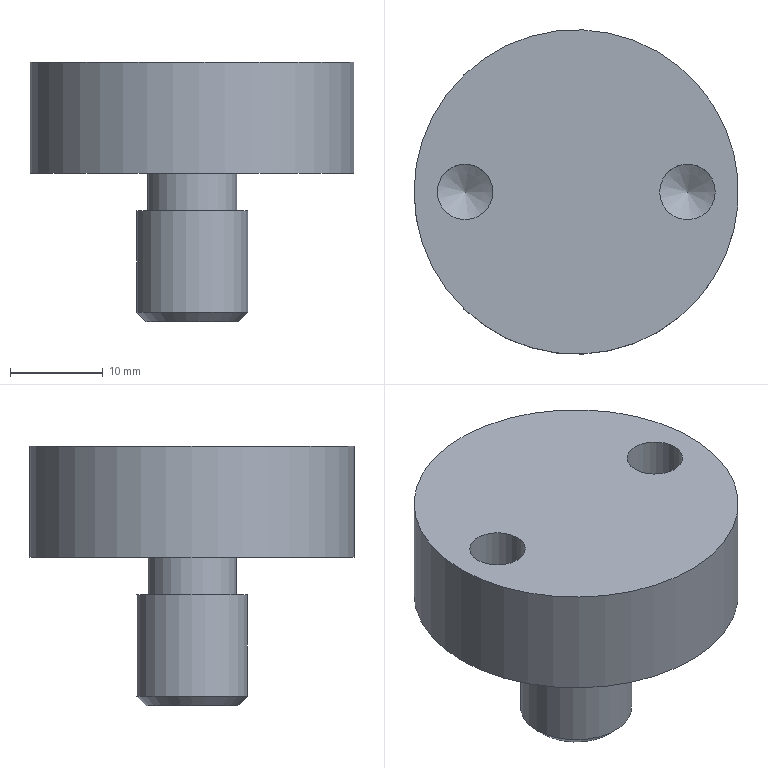Part | NX | features DATUM_CSYS 3, SIMPLE HOLE 2, SKETCH 2, CHAMFER 1, HOLE PACKAGE 1, SWP104 1, SYMBOLIC_THREAD 1 | 1 solid | 12 faces | box 35 x 35 x 28 mm | volume 12801 mm3 | cylinder 5 | plane 4 | cone 3 | commonest cylinder face diameters 6 x2 9.6 x1 12 x1 35 x1
STEP:
#1=CARTESIAN_POINT('',(-5.,0.,-28.));
#2=VERTEX_POINT('',#1);
#3=CARTESIAN_POINT('',(0.,0.,-28.));
#4=DIRECTION('',(0.,0.,-1.));
#5=DIRECTION('',(-1.,0.,0.));
#6=AXIS2_PLACEMENT_3D('',#3,#4,#5);
#7=CIRCLE('',#6,5.);
#8=EDGE_CURVE('',#2,#2,#7,.T.);
#9=ORIENTED_EDGE('',*,*,#8,.T.);
#10=EDGE_LOOP('',(#9));
#11=FACE_BOUND('',#10,.T.);
#12=CARTESIAN_POINT('',(0.,0.,-28.));
#13=DIRECTION('',(0.,0.,-1.));
#14=DIRECTION('',(-1.,0.,0.));
#15=AXIS2_PLACEMENT_3D('',#12,#13,#14);
#16=PLANE('',#15);
#17=ADVANCED_FACE('',(#11),#16,.T.);
#18=CARTESIAN_POINT('',(-6.,0.,-27.));
#19=VERTEX_POINT('',#18);
#20=CARTESIAN_POINT('',(0.,0.,-27.));
#21=DIRECTION('',(0.,0.,-1.));
#22=DIRECTION('',(-1.,0.,0.));
#23=AXIS2_PLACEMENT_3D('',#20,#21,#22);
#24=CIRCLE('',#23,6.);
#25=EDGE_CURVE('',#19,#19,#24,.F.);
#26=ORIENTED_EDGE('',*,*,#25,.T.);
#27=EDGE_LOOP('',(#26));
#28=FACE_BOUND('',#27,.T.);
#29=CARTESIAN_POINT('',(-6.,0.,-16.));
#30=VERTEX_POINT('',#29);
#31=CARTESIAN_POINT('',(0.,0.,-16.));
#32=DIRECTION('',(0.,0.,-1.));
#33=DIRECTION('',(-1.,0.,0.));
#34=AXIS2_PLACEMENT_3D('',#31,#32,#33);
#35=CIRCLE('',#34,6.);
#36=EDGE_CURVE('',#30,#30,#35,.T.);
#37=ORIENTED_EDGE('',*,*,#36,.T.);
#38=EDGE_LOOP('',(#37));
#39=FACE_BOUND('',#38,.T.);
#40=CARTESIAN_POINT('',(0.,0.,0.));
#41=DIRECTION('',(0.,0.,-1.));
#42=DIRECTION('',(-1.,0.,0.));
#43=AXIS2_PLACEMENT_3D('',#40,#41,#42);
#44=CYLINDRICAL_SURFACE('',#43,6.);
#45=ADVANCED_FACE('',(#28,#39),#44,.T.);
#46=CARTESIAN_POINT('',(-4.8,0.,-16.));
#47=VERTEX_POINT('',#46);
#48=CARTESIAN_POINT('',(0.,0.,-16.));
#49=DIRECTION('',(0.,0.,-1.));
#50=DIRECTION('',(-1.,0.,0.));
#51=AXIS2_PLACEMENT_3D('',#48,#49,#50);
#52=CIRCLE('',#51,4.8);
#53=EDGE_CURVE('',#47,#47,#52,.T.);
#54=ORIENTED_EDGE('',*,*,#53,.T.);
#55=EDGE_LOOP('',(#54));
#56=FACE_BOUND('',#55,.T.);
#57=ORIENTED_EDGE('',*,*,#36,.F.);
#58=EDGE_LOOP('',(#57));
#59=FACE_BOUND('',#58,.T.);
#60=CARTESIAN_POINT('',(6.,0.,-16.));
#61=DIRECTION('',(0.,0.,1.));
#62=DIRECTION('',(1.,0.,0.));
#63=AXIS2_PLACEMENT_3D('',#60,#61,#62);
#64=PLANE('',#63);
#65=ADVANCED_FACE('',(#56,#59),#64,.T.);
#66=CARTESIAN_POINT('',(-4.8,0.,-12.));
#67=VERTEX_POINT('',#66);
#68=CARTESIAN_POINT('',(0.,0.,-12.));
#69=DIRECTION('',(0.,0.,-1.));
#70=DIRECTION('',(-1.,0.,0.));
#71=AXIS2_PLACEMENT_3D('',#68,#69,#70);
#72=CIRCLE('',#71,4.8);
#73=EDGE_CURVE('',#67,#67,#72,.T.);
#74=ORIENTED_EDGE('',*,*,#73,.T.);
#75=EDGE_LOOP('',(#74));
#76=FACE_BOUND('',#75,.T.);
#77=ORIENTED_EDGE('',*,*,#53,.F.);
#78=EDGE_LOOP('',(#77));
#79=FACE_BOUND('',#78,.T.);
#80=CARTESIAN_POINT('',(0.,0.,0.));
#81=DIRECTION('',(0.,0.,-1.));
#82=DIRECTION('',(-1.,0.,0.));
#83=AXIS2_PLACEMENT_3D('',#80,#81,#82);
#84=CYLINDRICAL_SURFACE('',#83,4.8);
#85=ADVANCED_FACE('',(#76,#79),#84,.T.);
#86=CARTESIAN_POINT('',(-17.5,0.,-12.));
#87=VERTEX_POINT('',#86);
#88=CARTESIAN_POINT('',(0.,0.,-12.));
#89=DIRECTION('',(0.,0.,-1.));
#90=DIRECTION('',(-1.,0.,0.));
#91=AXIS2_PLACEMENT_3D('',#88,#89,#90);
#92=CIRCLE('',#91,17.5);
#93=EDGE_CURVE('',#87,#87,#92,.T.);
#94=ORIENTED_EDGE('',*,*,#93,.T.);
#95=EDGE_LOOP('',(#94));
#96=FACE_BOUND('',#95,.T.);
#97=ORIENTED_EDGE('',*,*,#73,.F.);
#98=EDGE_LOOP('',(#97));
#99=FACE_BOUND('',#98,.T.);
#100=CARTESIAN_POINT('',(4.8,0.,-12.));
#101=DIRECTION('',(0.,0.,-1.));
#102=DIRECTION('',(-1.,0.,0.));
#103=AXIS2_PLACEMENT_3D('',#100,#101,#102);
#104=PLANE('',#103);
#105=ADVANCED_FACE('',(#96,#99),#104,.T.);
#106=CARTESIAN_POINT('',(-17.5,0.,0.));
#107=VERTEX_POINT('',#106);
#108=CARTESIAN_POINT('',(0.,0.,0.));
#109=DIRECTION('',(0.,0.,-1.));
#110=DIRECTION('',(-1.,0.,0.));
#111=AXIS2_PLACEMENT_3D('',#108,#109,#110);
#112=CIRCLE('',#111,17.5);
#113=EDGE_CURVE('',#107,#107,#112,.T.);
#114=ORIENTED_EDGE('',*,*,#113,.T.);
#115=EDGE_LOOP('',(#114));
#116=FACE_BOUND('',#115,.T.);
#117=ORIENTED_EDGE('',*,*,#93,.F.);
#118=EDGE_LOOP('',(#117));
#119=FACE_BOUND('',#118,.T.);
#120=CARTESIAN_POINT('',(0.,0.,0.));
#121=DIRECTION('',(0.,0.,-1.));
#122=DIRECTION('',(-1.,0.,0.));
#123=AXIS2_PLACEMENT_3D('',#120,#121,#122);
#124=CYLINDRICAL_SURFACE('',#123,17.5);
#125=ADVANCED_FACE('',(#116,#119),#124,.T.);
#126=CARTESIAN_POINT('',(9.,0.,0.));
#127=VERTEX_POINT('',#126);
#128=CARTESIAN_POINT('',(12.,0.,0.));
#129=DIRECTION('',(0.,0.,-1.));
#130=DIRECTION('',(-1.,0.,0.));
#131=AXIS2_PLACEMENT_3D('',#128,#129,#130);
#132=CIRCLE('',#131,3.);
#133=EDGE_CURVE('',#127,#127,#132,.T.);
#134=ORIENTED_EDGE('',*,*,#133,.T.);
#135=EDGE_LOOP('',(#134));
#136=FACE_BOUND('',#135,.T.);
#137=CARTESIAN_POINT('',(-15.,0.,0.));
#138=VERTEX_POINT('',#137);
#139=CARTESIAN_POINT('',(-12.,0.,0.));
#140=DIRECTION('',(0.,0.,-1.));
#141=DIRECTION('',(-1.,0.,0.));
#142=AXIS2_PLACEMENT_3D('',#139,#140,#141);
#143=CIRCLE('',#142,3.);
#144=EDGE_CURVE('',#138,#138,#143,.T.);
#145=ORIENTED_EDGE('',*,*,#144,.T.);
#146=EDGE_LOOP('',(#145));
#147=FACE_BOUND('',#146,.T.);
#148=ORIENTED_EDGE('',*,*,#113,.F.);
#149=EDGE_LOOP('',(#148));
#150=FACE_BOUND('',#149,.T.);
#151=CARTESIAN_POINT('',(17.5,0.,0.));
#152=DIRECTION('',(0.,0.,1.));
#153=DIRECTION('',(1.,0.,0.));
#154=AXIS2_PLACEMENT_3D('',#151,#152,#153);
#155=PLANE('',#154);
#156=ADVANCED_FACE('',(#136,#147,#150),#155,.T.);
#157=CARTESIAN_POINT('',(-15.,0.,-6.));
#158=VERTEX_POINT('',#157);
#159=CARTESIAN_POINT('',(-12.,0.,-6.));
#160=DIRECTION('',(0.,0.,-1.));
#161=DIRECTION('',(-1.,0.,0.));
#162=AXIS2_PLACEMENT_3D('',#159,#160,#161);
#163=CIRCLE('',#162,3.);
#164=EDGE_CURVE('',#158,#158,#163,.F.);
#165=ORIENTED_EDGE('',*,*,#164,.T.);
#166=EDGE_LOOP('',(#165));
#167=FACE_BOUND('',#166,.T.);
#168=CARTESIAN_POINT('',(-12.,0.,-7.803));
#169=VERTEX_POINT('',#168);
#170=VERTEX_LOOP('',#169);
#171=FACE_BOUND('',#170,.T.);
#172=CARTESIAN_POINT('',(-12.,0.,-6.));
#173=DIRECTION('',(0.,0.,1.));
#174=DIRECTION('',(1.,0.,0.));
#175=AXIS2_PLACEMENT_3D('',#172,#173,#174);
#176=CONICAL_SURFACE('',#175,3.,1.03);
#177=ADVANCED_FACE('',(#167,#171),#176,.F.);
#178=ORIENTED_EDGE('',*,*,#164,.F.);
#179=EDGE_LOOP('',(#178));
#180=FACE_BOUND('',#179,.T.);
#181=ORIENTED_EDGE('',*,*,#144,.F.);
#182=EDGE_LOOP('',(#181));
#183=FACE_BOUND('',#182,.T.);
#184=CARTESIAN_POINT('',(-12.,0.,0.));
#185=DIRECTION('',(0.,0.,-1.));
#186=DIRECTION('',(-1.,0.,0.));
#187=AXIS2_PLACEMENT_3D('',#184,#185,#186);
#188=CYLINDRICAL_SURFACE('',#187,3.);
#189=ADVANCED_FACE('',(#180,#183),#188,.F.);
#190=CARTESIAN_POINT('',(9.,0.,-6.));
#191=VERTEX_POINT('',#190);
#192=CARTESIAN_POINT('',(12.,0.,-6.));
#193=DIRECTION('',(0.,0.,-1.));
#194=DIRECTION('',(-1.,0.,0.));
#195=AXIS2_PLACEMENT_3D('',#192,#193,#194);
#196=CIRCLE('',#195,3.);
#197=EDGE_CURVE('',#191,#191,#196,.F.);
#198=ORIENTED_EDGE('',*,*,#197,.T.);
#199=EDGE_LOOP('',(#198));
#200=FACE_BOUND('',#199,.T.);
#201=CARTESIAN_POINT('',(12.,0.,-7.803));
#202=VERTEX_POINT('',#201);
#203=VERTEX_LOOP('',#202);
#204=FACE_BOUND('',#203,.T.);
#205=CARTESIAN_POINT('',(12.,0.,-6.));
#206=DIRECTION('',(0.,0.,1.));
#207=DIRECTION('',(1.,0.,0.));
#208=AXIS2_PLACEMENT_3D('',#205,#206,#207);
#209=CONICAL_SURFACE('',#208,3.,1.03);
#210=ADVANCED_FACE('',(#200,#204),#209,.F.);
#211=ORIENTED_EDGE('',*,*,#197,.F.);
#212=EDGE_LOOP('',(#211));
#213=FACE_BOUND('',#212,.T.);
#214=ORIENTED_EDGE('',*,*,#133,.F.);
#215=EDGE_LOOP('',(#214));
#216=FACE_BOUND('',#215,.T.);
#217=CARTESIAN_POINT('',(12.,0.,0.));
#218=DIRECTION('',(0.,0.,-1.));
#219=DIRECTION('',(-1.,0.,0.));
#220=AXIS2_PLACEMENT_3D('',#217,#218,#219);
#221=CYLINDRICAL_SURFACE('',#220,3.);
#222=ADVANCED_FACE('',(#213,#216),#221,.F.);
#223=ORIENTED_EDGE('',*,*,#25,.F.);
#224=EDGE_LOOP('',(#223));
#225=FACE_BOUND('',#224,.T.);
#226=ORIENTED_EDGE('',*,*,#8,.F.);
#227=EDGE_LOOP('',(#226));
#228=FACE_BOUND('',#227,.T.);
#229=CARTESIAN_POINT('',(0.,0.,-28.));
#230=DIRECTION('',(0.,0.,1.));
#231=DIRECTION('',(1.,0.,0.));
#232=AXIS2_PLACEMENT_3D('',#229,#230,#231);
#233=CONICAL_SURFACE('',#232,5.,0.7854);
#234=ADVANCED_FACE('',(#225,#228),#233,.T.);
#235=CLOSED_SHELL('',(#17,#45,#65,#85,#105,#125,#156,#177,#189,#210,#222,#234));
#236=MANIFOLD_SOLID_BREP('',#235);
#237=(LENGTH_UNIT()NAMED_UNIT(*)SI_UNIT(.MILLI.,.METRE.));
#238=UNCERTAINTY_MEASURE_WITH_UNIT(LENGTH_MEASURE(0.00001),#237,'','');
#239=(NAMED_UNIT(*)PLANE_ANGLE_UNIT()SI_UNIT($,.RADIAN.));
#240=(NAMED_UNIT(*)SI_UNIT($,.STERADIAN.)SOLID_ANGLE_UNIT());
#241=(GEOMETRIC_REPRESENTATION_CONTEXT(3)GLOBAL_UNCERTAINTY_ASSIGNED_CONTEXT((#238))GLOBAL_UNIT_ASSIGNED_CONTEXT((#237,#239,#240))REPRESENTATION_CONTEXT('',''));
#242=ADVANCED_BREP_SHAPE_REPRESENTATION('',(#236),#241);